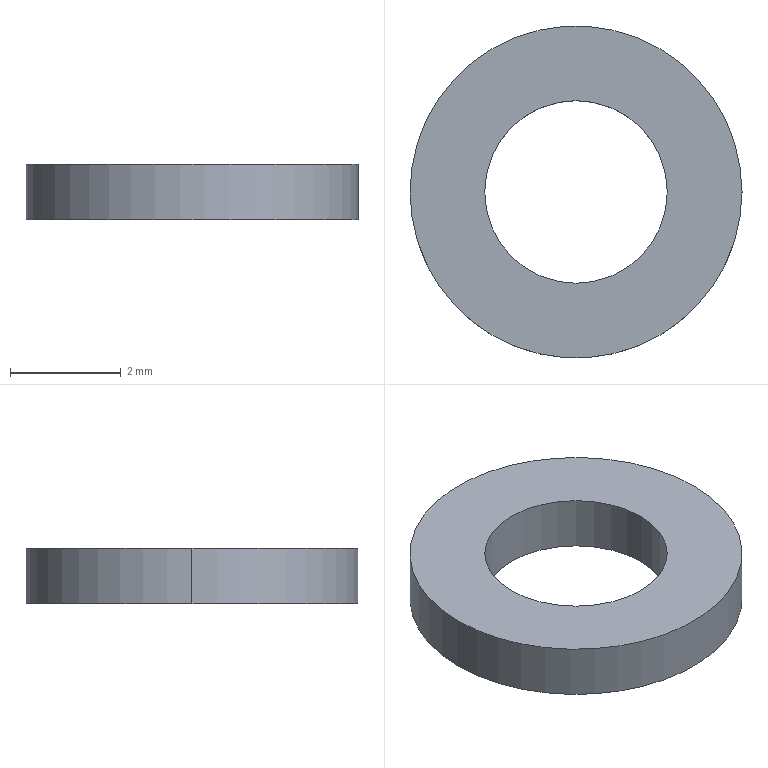Part | SolidWorks | features BaseBody 1 | 1 solid | 6 faces | box 6 x 6 x 1 mm | volume 19.721 mm3 | cylinder 4 | plane 2 | commonest cylinder face diameters 3.3 x2 6 x2
STEP:
#1=CARTESIAN_POINT('',(-1.65,0.,-1.));
#2=VERTEX_POINT('',#1);
#3=CARTESIAN_POINT('',(1.65,0.,-1.));
#4=VERTEX_POINT('',#3);
#5=CARTESIAN_POINT('',(0.,0.,-1.));
#6=DIRECTION('',(0.,0.,1.));
#7=DIRECTION('',(1.,0.,0.));
#8=AXIS2_PLACEMENT_3D('',#5,#6,#7);
#9=CIRCLE('',#8,1.65);
#10=EDGE_CURVE('',#2,#4,#9,.T.);
#11=ORIENTED_EDGE('',*,*,#10,.F.);
#12=CARTESIAN_POINT('',(-1.65,0.,0.));
#13=VERTEX_POINT('',#12);
#14=CARTESIAN_POINT('',(-1.65,0.,-1.));
#15=DIRECTION('',(0.,0.,1.));
#16=VECTOR('',#15,1000.);
#17=LINE('',#14,#16);
#18=EDGE_CURVE('',#2,#13,#17,.T.);
#19=ORIENTED_EDGE('',*,*,#18,.T.);
#20=CARTESIAN_POINT('',(1.65,0.,0.));
#21=VERTEX_POINT('',#20);
#22=CARTESIAN_POINT('',(0.,0.,0.));
#23=DIRECTION('',(0.,0.,-1.));
#24=DIRECTION('',(1.,0.,0.));
#25=AXIS2_PLACEMENT_3D('',#22,#23,#24);
#26=CIRCLE('',#25,1.65);
#27=EDGE_CURVE('',#21,#13,#26,.T.);
#28=ORIENTED_EDGE('',*,*,#27,.F.);
#29=CARTESIAN_POINT('',(1.65,0.,-1.));
#30=DIRECTION('',(0.,0.,1.));
#31=VECTOR('',#30,1000.);
#32=LINE('',#29,#31);
#33=EDGE_CURVE('',#4,#21,#32,.T.);
#34=ORIENTED_EDGE('',*,*,#33,.F.);
#35=EDGE_LOOP('',(#11,#19,#28,#34));
#36=FACE_OUTER_BOUND('',#35,.T.);
#37=CARTESIAN_POINT('',(0.,0.,-1.));
#38=DIRECTION('',(0.,0.,1.));
#39=DIRECTION('',(1.,0.,0.));
#40=AXIS2_PLACEMENT_3D('',#37,#38,#39);
#41=CYLINDRICAL_SURFACE('',#40,1.65);
#42=ADVANCED_FACE('',(#36),#41,.F.);
#43=CARTESIAN_POINT('',(3.,0.,-1.));
#44=VERTEX_POINT('',#43);
#45=CARTESIAN_POINT('',(-3.,0.,-1.));
#46=VERTEX_POINT('',#45);
#47=CARTESIAN_POINT('',(0.,0.,-1.));
#48=DIRECTION('',(0.,0.,1.));
#49=DIRECTION('',(1.,0.,0.));
#50=AXIS2_PLACEMENT_3D('',#47,#48,#49);
#51=CIRCLE('',#50,3.);
#52=EDGE_CURVE('',#44,#46,#51,.T.);
#53=ORIENTED_EDGE('',*,*,#52,.T.);
#54=CARTESIAN_POINT('',(-3.,0.,0.));
#55=VERTEX_POINT('',#54);
#56=CARTESIAN_POINT('',(-3.,0.,-1.));
#57=DIRECTION('',(0.,0.,1.));
#58=VECTOR('',#57,1000.);
#59=LINE('',#56,#58);
#60=EDGE_CURVE('',#46,#55,#59,.T.);
#61=ORIENTED_EDGE('',*,*,#60,.T.);
#62=CARTESIAN_POINT('',(3.,0.,0.));
#63=VERTEX_POINT('',#62);
#64=CARTESIAN_POINT('',(0.,0.,0.));
#65=DIRECTION('',(0.,0.,1.));
#66=DIRECTION('',(1.,0.,0.));
#67=AXIS2_PLACEMENT_3D('',#64,#65,#66);
#68=CIRCLE('',#67,3.);
#69=EDGE_CURVE('',#63,#55,#68,.T.);
#70=ORIENTED_EDGE('',*,*,#69,.F.);
#71=CARTESIAN_POINT('',(3.,0.,-1.));
#72=DIRECTION('',(0.,0.,1.));
#73=VECTOR('',#72,1000.);
#74=LINE('',#71,#73);
#75=EDGE_CURVE('',#44,#63,#74,.T.);
#76=ORIENTED_EDGE('',*,*,#75,.F.);
#77=EDGE_LOOP('',(#53,#61,#70,#76));
#78=FACE_OUTER_BOUND('',#77,.T.);
#79=CARTESIAN_POINT('',(0.,0.,-1.));
#80=DIRECTION('',(0.,0.,1.));
#81=DIRECTION('',(1.,0.,0.));
#82=AXIS2_PLACEMENT_3D('',#79,#80,#81);
#83=CYLINDRICAL_SURFACE('',#82,3.);
#84=ADVANCED_FACE('',(#78),#83,.T.);
#85=ORIENTED_EDGE('',*,*,#27,.T.);
#86=CARTESIAN_POINT('',(0.,0.,0.));
#87=DIRECTION('',(0.,0.,-1.));
#88=DIRECTION('',(1.,0.,0.));
#89=AXIS2_PLACEMENT_3D('',#86,#87,#88);
#90=CIRCLE('',#89,1.65);
#91=EDGE_CURVE('',#13,#21,#90,.T.);
#92=ORIENTED_EDGE('',*,*,#91,.T.);
#93=EDGE_LOOP('',(#85,#92));
#94=FACE_BOUND('',#93,.T.);
#95=ORIENTED_EDGE('',*,*,#69,.T.);
#96=CARTESIAN_POINT('',(0.,0.,0.));
#97=DIRECTION('',(0.,0.,1.));
#98=DIRECTION('',(1.,0.,0.));
#99=AXIS2_PLACEMENT_3D('',#96,#97,#98);
#100=CIRCLE('',#99,3.);
#101=EDGE_CURVE('',#55,#63,#100,.T.);
#102=ORIENTED_EDGE('',*,*,#101,.T.);
#103=EDGE_LOOP('',(#95,#102));
#104=FACE_OUTER_BOUND('',#103,.T.);
#105=CARTESIAN_POINT('',(1.65,0.,0.));
#106=DIRECTION('',(0.,0.,1.));
#107=DIRECTION('',(1.,0.,0.));
#108=AXIS2_PLACEMENT_3D('',#105,#106,#107);
#109=PLANE('',#108);
#110=ADVANCED_FACE('',(#94,#104),#109,.T.);
#111=ORIENTED_EDGE('',*,*,#18,.F.);
#112=CARTESIAN_POINT('',(0.,0.,-1.));
#113=DIRECTION('',(0.,0.,1.));
#114=DIRECTION('',(1.,0.,0.));
#115=AXIS2_PLACEMENT_3D('',#112,#113,#114);
#116=CIRCLE('',#115,1.65);
#117=EDGE_CURVE('',#4,#2,#116,.T.);
#118=ORIENTED_EDGE('',*,*,#117,.F.);
#119=ORIENTED_EDGE('',*,*,#33,.T.);
#120=ORIENTED_EDGE('',*,*,#91,.F.);
#121=EDGE_LOOP('',(#111,#118,#119,#120));
#122=FACE_OUTER_BOUND('',#121,.T.);
#123=CARTESIAN_POINT('',(0.,0.,-1.));
#124=DIRECTION('',(0.,0.,1.));
#125=DIRECTION('',(1.,0.,0.));
#126=AXIS2_PLACEMENT_3D('',#123,#124,#125);
#127=CYLINDRICAL_SURFACE('',#126,1.65);
#128=ADVANCED_FACE('',(#122),#127,.F.);
#129=ORIENTED_EDGE('',*,*,#60,.F.);
#130=CARTESIAN_POINT('',(0.,0.,-1.));
#131=DIRECTION('',(0.,0.,1.));
#132=DIRECTION('',(1.,0.,0.));
#133=AXIS2_PLACEMENT_3D('',#130,#131,#132);
#134=CIRCLE('',#133,3.);
#135=EDGE_CURVE('',#46,#44,#134,.T.);
#136=ORIENTED_EDGE('',*,*,#135,.T.);
#137=ORIENTED_EDGE('',*,*,#75,.T.);
#138=ORIENTED_EDGE('',*,*,#101,.F.);
#139=EDGE_LOOP('',(#129,#136,#137,#138));
#140=FACE_OUTER_BOUND('',#139,.T.);
#141=CARTESIAN_POINT('',(0.,0.,-1.));
#142=DIRECTION('',(0.,0.,1.));
#143=DIRECTION('',(1.,0.,0.));
#144=AXIS2_PLACEMENT_3D('',#141,#142,#143);
#145=CYLINDRICAL_SURFACE('',#144,3.);
#146=ADVANCED_FACE('',(#140),#145,.T.);
#147=ORIENTED_EDGE('',*,*,#52,.F.);
#148=ORIENTED_EDGE('',*,*,#135,.F.);
#149=EDGE_LOOP('',(#147,#148));
#150=FACE_OUTER_BOUND('',#149,.T.);
#151=ORIENTED_EDGE('',*,*,#117,.T.);
#152=ORIENTED_EDGE('',*,*,#10,.T.);
#153=EDGE_LOOP('',(#151,#152));
#154=FACE_BOUND('',#153,.T.);
#155=CARTESIAN_POINT('',(3.,0.,-1.));
#156=DIRECTION('',(0.,0.,-1.));
#157=DIRECTION('',(-1.,0.,0.));
#158=AXIS2_PLACEMENT_3D('',#155,#156,#157);
#159=PLANE('',#158);
#160=ADVANCED_FACE('',(#150,#154),#159,.T.);
#161=CLOSED_SHELL('',(#42,#84,#110,#128,#146,#160));
#162=MANIFOLD_SOLID_BREP('',#161);
#163=CARTESIAN_POINT('',(0.,0.,0.));
#164=DIRECTION('',(0.,0.,1.));
#165=DIRECTION('',(1.,0.,0.));
#166=AXIS2_PLACEMENT_3D('',#163,#164,#165);
#167=(LENGTH_UNIT()NAMED_UNIT(*)SI_UNIT(.MILLI.,.METRE.));
#168=UNCERTAINTY_MEASURE_WITH_UNIT(LENGTH_MEASURE(0.00001),#167,'','');
#169=(NAMED_UNIT(*)PLANE_ANGLE_UNIT()SI_UNIT($,.RADIAN.));
#170=(NAMED_UNIT(*)SI_UNIT($,.STERADIAN.)SOLID_ANGLE_UNIT());
#171=(GEOMETRIC_REPRESENTATION_CONTEXT(3)GLOBAL_UNCERTAINTY_ASSIGNED_CONTEXT((#168))GLOBAL_UNIT_ASSIGNED_CONTEXT((#167,#169,#170))REPRESENTATION_CONTEXT('',''));
#172=ADVANCED_BREP_SHAPE_REPRESENTATION('',(#162,#166),#171);